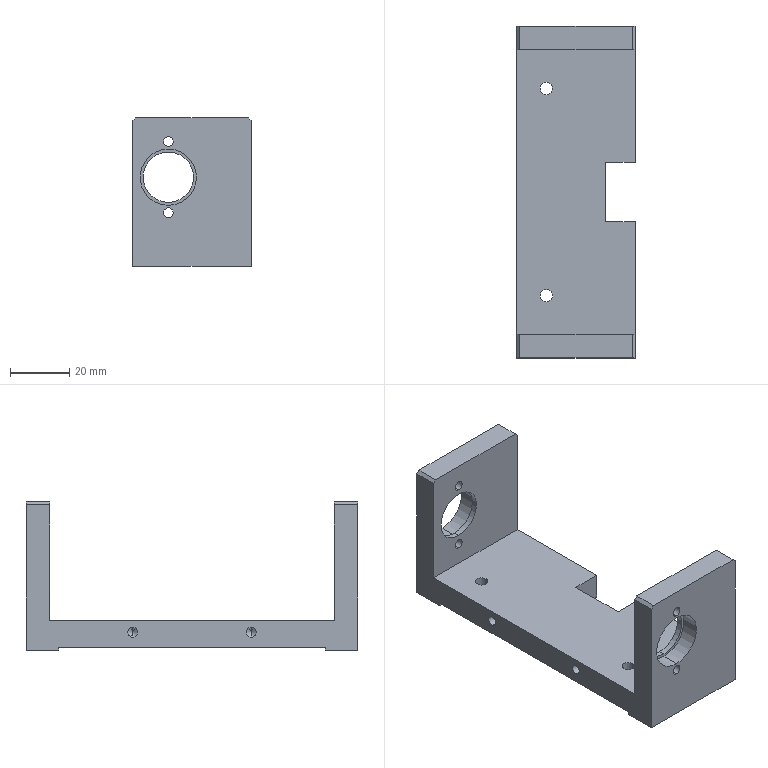Part | STEP file | 2050 Upper bearing mounting plate | 1 solid | 76 faces | box 40 x 112 x 50 mm | volume 59323 mm3 | cylinder 36 | plane 24 | cone 16 | commonest cylinder face diameters 3.3 x24 4.2 x4 17 x4 19 x4